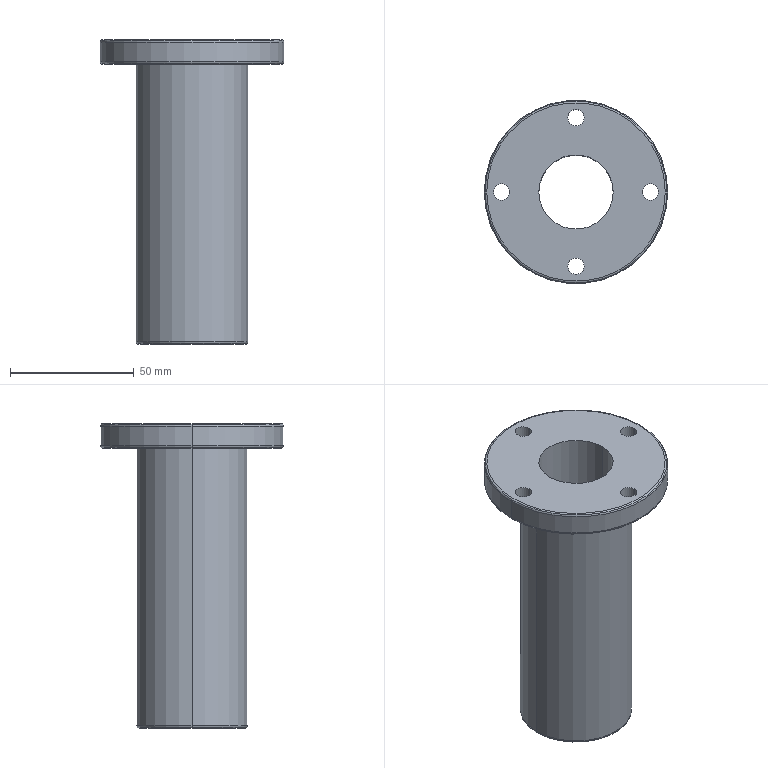Part | NX | features BREP 1 | 1 solid | 65 faces | box 74 x 74 x 123 mm | volume 134244 mm3 | plane 27 | cylinder 20 | torus 12 | cone 6 | commonest cylinder face diameters 6.6 x8 8.5 x6 30 x2 45 x2 74 x2